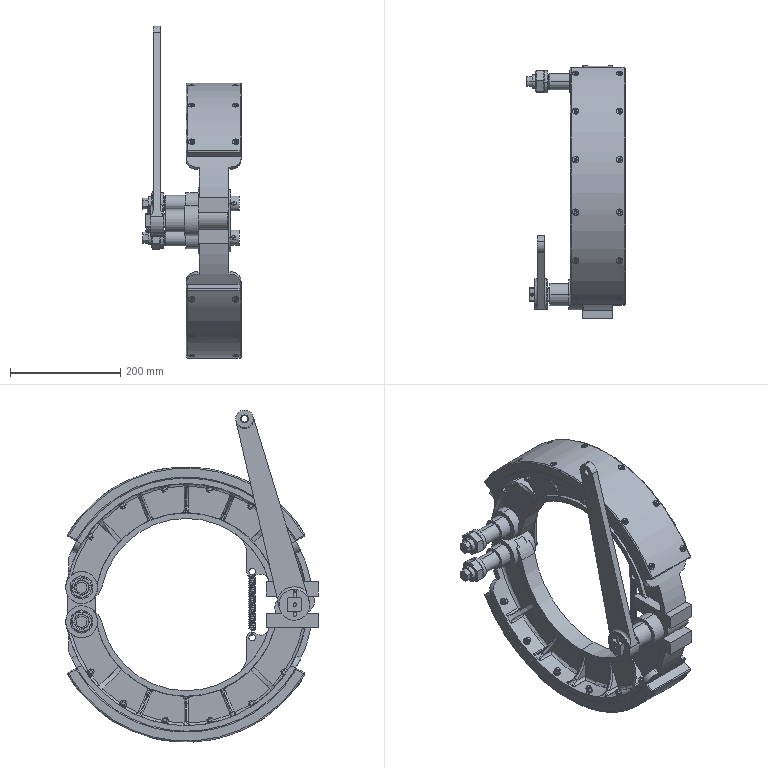Part | SolidWorks | features ReferencePattern 44, MateUpdatePoint 4, LocalCirPattern 1, LocalLPattern 1, RefAxis 1 | 113 solids | 3172 faces | volume 5849536 mm3 | cylinder 1545 | plane 801 | cone 596 | torus 128 | spline 86 | sphere 16 | commonest cylinder face diameters 0.4 x384 1.57 x216 6 x180 5.72 x144 8 x96 9.205 x72